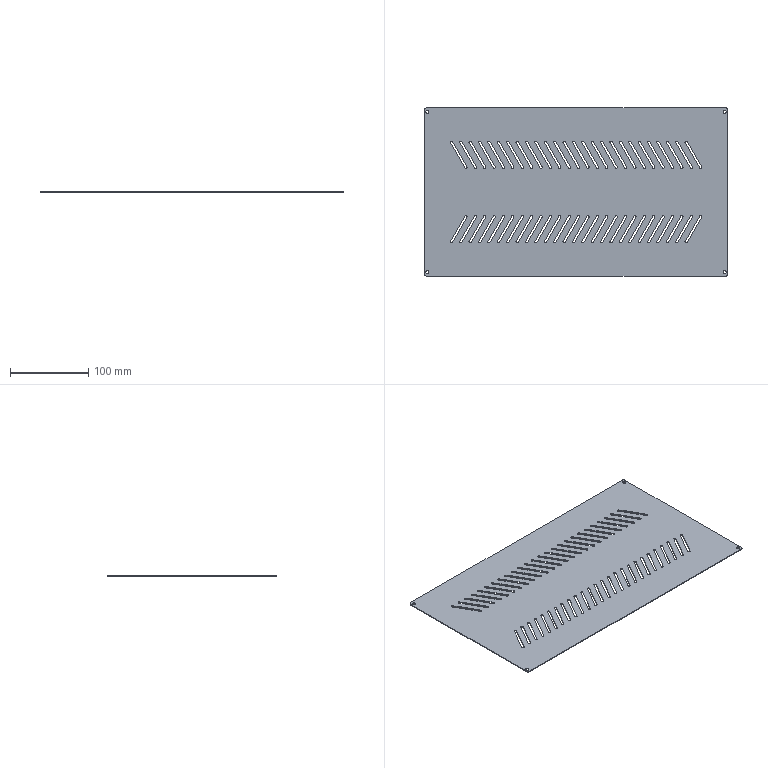Part | SolidWorks | features BaseBody 1 | 1 solid | 278 faces | box 388 x 215 x 1 mm | volume 77225 mm3 | cylinder 168 | plane 110 | commonest cylinder face diameters 3 x156 4 x10 6 x2